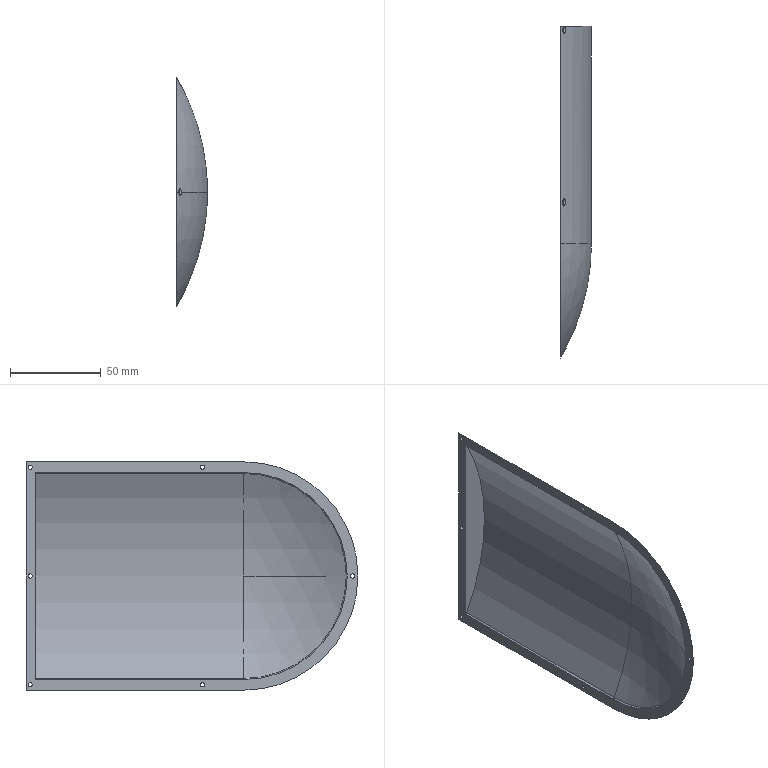Part | SolidWorks | features ICE 3, Cut 1, Fillet 1, OffsetRefSurface 1, Revolution 1, SewRefSurface 1, Shell 1 | 1 solid | 44 faces | box 17 x 182.936 x 125.873 mm | volume 49131 mm3 | cylinder 28 | plane 11 | sphere 4 | torus 1 | commonest cylinder face diameters 2.3 x12 4 x11 2 x2 114.129 x1 246 x1 250 x1